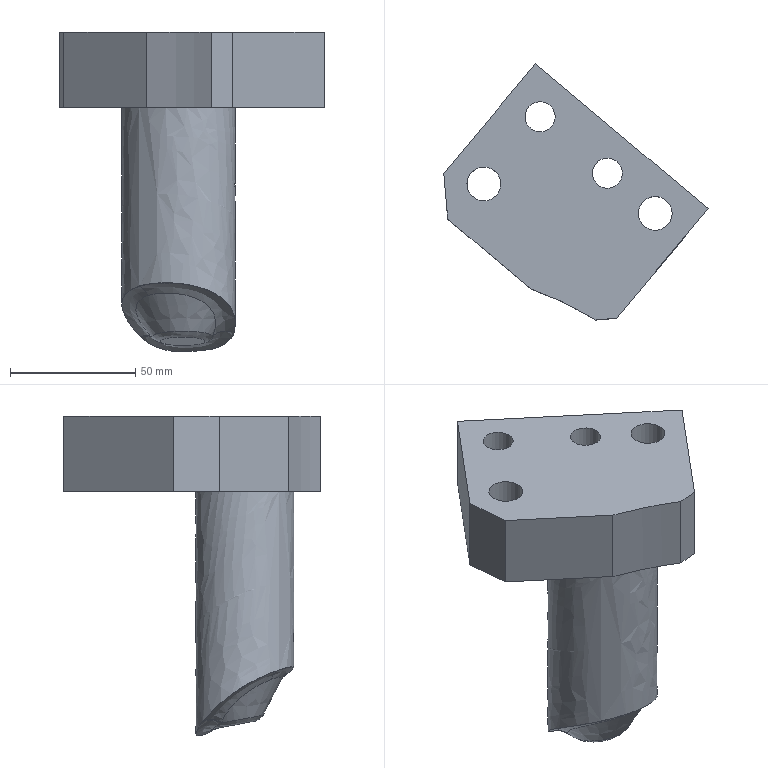Part | NX | features solid 2 | 1 solid | 27 faces | box 105.583 x 102.258 x 127.556 mm | volume 283644 mm3 | plane 11 | spline 10 | cylinder 6 | commonest cylinder face diameters 12 x2 13.5 x2 19.5 x2